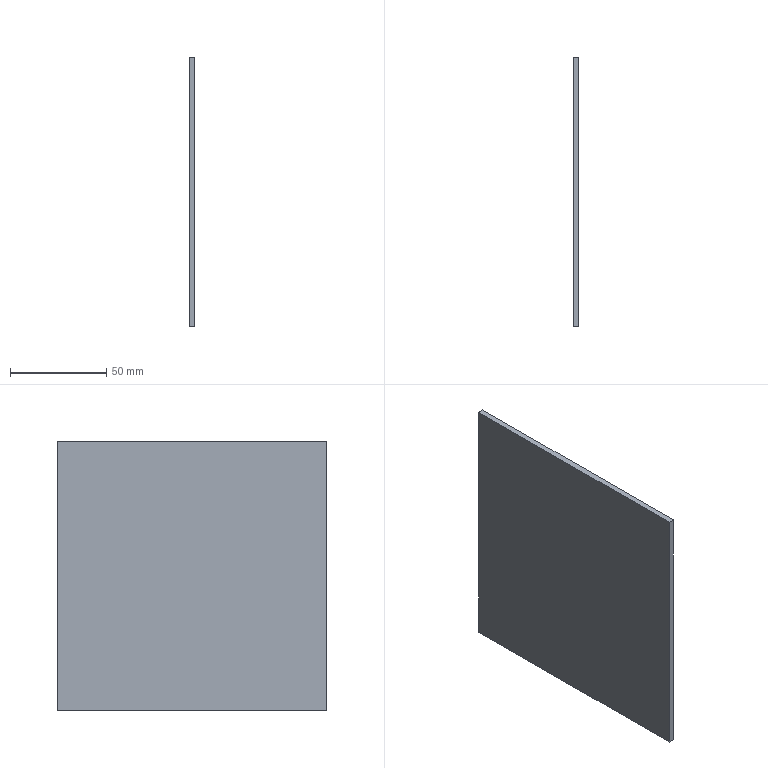Part | STEP file | Positioning_id1514_x_t | 1 solid | 6 faces | box 3 x 140 x 140 mm | volume 58800 mm3 | plane 6
STEP:
#1=CARTESIAN_POINT('',(0.,0.,0.));
#2=DIRECTION('',(0.,0.,1.));
#3=DIRECTION('',(1.,0.,0.));
#4=AXIS2_PLACEMENT_3D('',#1,#2,#3);
#5=CARTESIAN_POINT('',(-1013.002,-340.,368.995));
#6=VERTEX_POINT('',#5);
#7=CARTESIAN_POINT('',(-1010.002,-340.,368.995));
#8=VERTEX_POINT('',#7);
#9=CARTESIAN_POINT('',(-1013.002,-340.,368.995));
#10=DIRECTION('',(1.,0.,0.));
#11=VECTOR('',#10,1.);
#12=LINE('',#9,#11);
#13=CARTESIAN_POINT('',(-1018.002,-340.,283.995));
#14=DIRECTION('',(0.,1.,0.));
#15=DIRECTION('',(1.,0.,0.));
#16=AXIS2_PLACEMENT_3D('',#13,#14,#15);
#17=PLANE('',#16);
#18=CARTESIAN_POINT('',(5.,-85.));
#19=DIRECTION('',(1.,0.));
#20=VECTOR('',#19,1.);
#21=LINE('',#18,#20);
#22=(GEOMETRIC_REPRESENTATION_CONTEXT(2)PARAMETRIC_REPRESENTATION_CONTEXT()REPRESENTATION_CONTEXT('',''));
#23=DEFINITIONAL_REPRESENTATION('',(#21),#22);
#24=PCURVE('',#17,#23);
#25=CARTESIAN_POINT('',(-1018.002,-428.,368.995));
#26=DIRECTION('',(0.,0.,1.));
#27=DIRECTION('',(1.,0.,0.));
#28=AXIS2_PLACEMENT_3D('',#25,#26,#27);
#29=PLANE('',#28);
#30=CARTESIAN_POINT('',(5.,88.));
#31=DIRECTION('',(1.,0.));
#32=VECTOR('',#31,1.);
#33=LINE('',#30,#32);
#34=(GEOMETRIC_REPRESENTATION_CONTEXT(2)PARAMETRIC_REPRESENTATION_CONTEXT()REPRESENTATION_CONTEXT('',''));
#35=DEFINITIONAL_REPRESENTATION('',(#33),#34);
#36=PCURVE('',#29,#35);
#37=SURFACE_CURVE('',#12,(#24,#36),.PCURVE_S1.);
#38=EDGE_CURVE('',#6,#8,#37,.T.);
#39=ORIENTED_EDGE('',*,*,#38,.T.);
#40=CARTESIAN_POINT('',(-1010.002,-340.,228.995));
#41=VERTEX_POINT('',#40);
#42=CARTESIAN_POINT('',(-1010.002,-340.,368.995));
#43=DIRECTION('',(0.,0.,-1.));
#44=VECTOR('',#43,1.);
#45=LINE('',#42,#44);
#46=CARTESIAN_POINT('',(8.,-85.));
#47=DIRECTION('',(0.,1.));
#48=VECTOR('',#47,1.);
#49=LINE('',#46,#48);
#50=(GEOMETRIC_REPRESENTATION_CONTEXT(2)PARAMETRIC_REPRESENTATION_CONTEXT()REPRESENTATION_CONTEXT('',''));
#51=DEFINITIONAL_REPRESENTATION('',(#49),#50);
#52=PCURVE('',#17,#51);
#53=CARTESIAN_POINT('',(-1010.002,-480.,368.995));
#54=DIRECTION('',(1.,0.,0.));
#55=DIRECTION('',(0.,0.,-1.));
#56=AXIS2_PLACEMENT_3D('',#53,#54,#55);
#57=PLANE('',#56);
#58=CARTESIAN_POINT('',(0.,140.));
#59=DIRECTION('',(1.,0.));
#60=VECTOR('',#59,1.);
#61=LINE('',#58,#60);
#62=(GEOMETRIC_REPRESENTATION_CONTEXT(2)PARAMETRIC_REPRESENTATION_CONTEXT()REPRESENTATION_CONTEXT('',''));
#63=DEFINITIONAL_REPRESENTATION('',(#61),#62);
#64=PCURVE('',#57,#63);
#65=SURFACE_CURVE('',#45,(#52,#64),.PCURVE_S1.);
#66=EDGE_CURVE('',#8,#41,#65,.T.);
#67=ORIENTED_EDGE('',*,*,#66,.T.);
#68=CARTESIAN_POINT('',(-1013.002,-340.,228.995));
#69=VERTEX_POINT('',#68);
#70=CARTESIAN_POINT('',(-1013.002,-340.,228.995));
#71=DIRECTION('',(1.,0.,0.));
#72=VECTOR('',#71,1.);
#73=LINE('',#70,#72);
#74=CARTESIAN_POINT('',(5.,55.));
#75=DIRECTION('',(1.,0.));
#76=VECTOR('',#75,1.);
#77=LINE('',#74,#76);
#78=(GEOMETRIC_REPRESENTATION_CONTEXT(2)PARAMETRIC_REPRESENTATION_CONTEXT()REPRESENTATION_CONTEXT('',''));
#79=DEFINITIONAL_REPRESENTATION('',(#77),#78);
#80=PCURVE('',#17,#79);
#81=CARTESIAN_POINT('',(-1018.002,-428.,228.995));
#82=DIRECTION('',(0.,0.,-1.));
#83=DIRECTION('',(-1.,0.,0.));
#84=AXIS2_PLACEMENT_3D('',#81,#82,#83);
#85=PLANE('',#84);
#86=CARTESIAN_POINT('',(-5.,88.));
#87=DIRECTION('',(-1.,0.));
#88=VECTOR('',#87,1.);
#89=LINE('',#86,#88);
#90=(GEOMETRIC_REPRESENTATION_CONTEXT(2)PARAMETRIC_REPRESENTATION_CONTEXT()REPRESENTATION_CONTEXT('',''));
#91=DEFINITIONAL_REPRESENTATION('',(#89),#90);
#92=PCURVE('',#85,#91);
#93=SURFACE_CURVE('',#73,(#80,#92),.PCURVE_S1.);
#94=EDGE_CURVE('',#69,#41,#93,.T.);
#95=ORIENTED_EDGE('',*,*,#94,.F.);
#96=CARTESIAN_POINT('',(-1013.002,-340.,228.995));
#97=DIRECTION('',(0.,0.,1.));
#98=VECTOR('',#97,1.);
#99=LINE('',#96,#98);
#100=CARTESIAN_POINT('',(5.,55.));
#101=DIRECTION('',(0.,-1.));
#102=VECTOR('',#101,1.);
#103=LINE('',#100,#102);
#104=(GEOMETRIC_REPRESENTATION_CONTEXT(2)PARAMETRIC_REPRESENTATION_CONTEXT()REPRESENTATION_CONTEXT('',''));
#105=DEFINITIONAL_REPRESENTATION('',(#103),#104);
#106=PCURVE('',#17,#105);
#107=CARTESIAN_POINT('',(-1013.002,-428.,283.995));
#108=DIRECTION('',(-1.,0.,0.));
#109=DIRECTION('',(0.,0.,1.));
#110=AXIS2_PLACEMENT_3D('',#107,#108,#109);
#111=PLANE('',#110);
#112=CARTESIAN_POINT('',(-55.,88.));
#113=DIRECTION('',(1.,0.));
#114=VECTOR('',#113,1.);
#115=LINE('',#112,#114);
#116=(GEOMETRIC_REPRESENTATION_CONTEXT(2)PARAMETRIC_REPRESENTATION_CONTEXT()REPRESENTATION_CONTEXT('',''));
#117=DEFINITIONAL_REPRESENTATION('',(#115),#116);
#118=PCURVE('',#111,#117);
#119=SURFACE_CURVE('',#99,(#106,#118),.PCURVE_S1.);
#120=EDGE_CURVE('',#69,#6,#119,.T.);
#121=ORIENTED_EDGE('',*,*,#120,.T.);
#122=EDGE_LOOP('',(#39,#67,#95,#121));
#123=FACE_BOUND('',#122,.T.);
#124=ADVANCED_FACE('',(#123),#17,.T.);
#125=ORIENTED_EDGE('',*,*,#94,.T.);
#126=CARTESIAN_POINT('',(-1010.002,-480.,228.995));
#127=VERTEX_POINT('',#126);
#128=CARTESIAN_POINT('',(-1010.002,-340.,228.995));
#129=DIRECTION('',(0.,-1.,0.));
#130=VECTOR('',#129,1.);
#131=LINE('',#128,#130);
#132=CARTESIAN_POINT('',(-8.,88.));
#133=DIRECTION('',(0.,-1.));
#134=VECTOR('',#133,1.);
#135=LINE('',#132,#134);
#136=(GEOMETRIC_REPRESENTATION_CONTEXT(2)PARAMETRIC_REPRESENTATION_CONTEXT()REPRESENTATION_CONTEXT('',''));
#137=DEFINITIONAL_REPRESENTATION('',(#135),#136);
#138=PCURVE('',#85,#137);
#139=CARTESIAN_POINT('',(140.,140.));
#140=DIRECTION('',(0.,-1.));
#141=VECTOR('',#140,1.);
#142=LINE('',#139,#141);
#143=(GEOMETRIC_REPRESENTATION_CONTEXT(2)PARAMETRIC_REPRESENTATION_CONTEXT()REPRESENTATION_CONTEXT('',''));
#144=DEFINITIONAL_REPRESENTATION('',(#142),#143);
#145=PCURVE('',#57,#144);
#146=SURFACE_CURVE('',#131,(#138,#145),.PCURVE_S1.);
#147=EDGE_CURVE('',#41,#127,#146,.T.);
#148=ORIENTED_EDGE('',*,*,#147,.T.);
#149=CARTESIAN_POINT('',(-1013.002,-480.,228.995));
#150=VERTEX_POINT('',#149);
#151=CARTESIAN_POINT('',(-1013.002,-480.,228.995));
#152=DIRECTION('',(1.,0.,0.));
#153=VECTOR('',#152,1.);
#154=LINE('',#151,#153);
#155=CARTESIAN_POINT('',(-5.,-52.));
#156=DIRECTION('',(-1.,0.));
#157=VECTOR('',#156,1.);
#158=LINE('',#155,#157);
#159=(GEOMETRIC_REPRESENTATION_CONTEXT(2)PARAMETRIC_REPRESENTATION_CONTEXT()REPRESENTATION_CONTEXT('',''));
#160=DEFINITIONAL_REPRESENTATION('',(#158),#159);
#161=PCURVE('',#85,#160);
#162=CARTESIAN_POINT('',(-1018.002,-480.,283.995));
#163=DIRECTION('',(0.,-1.,0.));
#164=DIRECTION('',(-1.,0.,0.));
#165=AXIS2_PLACEMENT_3D('',#162,#163,#164);
#166=PLANE('',#165);
#167=CARTESIAN_POINT('',(-5.,55.));
#168=DIRECTION('',(-1.,0.));
#169=VECTOR('',#168,1.);
#170=LINE('',#167,#169);
#171=(GEOMETRIC_REPRESENTATION_CONTEXT(2)PARAMETRIC_REPRESENTATION_CONTEXT()REPRESENTATION_CONTEXT('',''));
#172=DEFINITIONAL_REPRESENTATION('',(#170),#171);
#173=PCURVE('',#166,#172);
#174=SURFACE_CURVE('',#154,(#161,#173),.PCURVE_S1.);
#175=EDGE_CURVE('',#150,#127,#174,.T.);
#176=ORIENTED_EDGE('',*,*,#175,.F.);
#177=CARTESIAN_POINT('',(-1013.002,-480.,228.995));
#178=DIRECTION('',(0.,1.,0.));
#179=VECTOR('',#178,1.);
#180=LINE('',#177,#179);
#181=CARTESIAN_POINT('',(-5.,-52.));
#182=DIRECTION('',(0.,1.));
#183=VECTOR('',#182,1.);
#184=LINE('',#181,#183);
#185=(GEOMETRIC_REPRESENTATION_CONTEXT(2)PARAMETRIC_REPRESENTATION_CONTEXT()REPRESENTATION_CONTEXT('',''));
#186=DEFINITIONAL_REPRESENTATION('',(#184),#185);
#187=PCURVE('',#85,#186);
#188=CARTESIAN_POINT('',(-55.,-52.));
#189=DIRECTION('',(0.,1.));
#190=VECTOR('',#189,1.);
#191=LINE('',#188,#190);
#192=(GEOMETRIC_REPRESENTATION_CONTEXT(2)PARAMETRIC_REPRESENTATION_CONTEXT()REPRESENTATION_CONTEXT('',''));
#193=DEFINITIONAL_REPRESENTATION('',(#191),#192);
#194=PCURVE('',#111,#193);
#195=SURFACE_CURVE('',#180,(#187,#194),.PCURVE_S1.);
#196=EDGE_CURVE('',#150,#69,#195,.T.);
#197=ORIENTED_EDGE('',*,*,#196,.T.);
#198=EDGE_LOOP('',(#125,#148,#176,#197));
#199=FACE_BOUND('',#198,.T.);
#200=ADVANCED_FACE('',(#199),#85,.T.);
#201=ORIENTED_EDGE('',*,*,#175,.T.);
#202=CARTESIAN_POINT('',(-1010.002,-480.,368.995));
#203=VERTEX_POINT('',#202);
#204=CARTESIAN_POINT('',(-1010.002,-480.,228.995));
#205=DIRECTION('',(0.,0.,1.));
#206=VECTOR('',#205,1.);
#207=LINE('',#204,#206);
#208=CARTESIAN_POINT('',(-8.,55.));
#209=DIRECTION('',(0.,-1.));
#210=VECTOR('',#209,1.);
#211=LINE('',#208,#210);
#212=(GEOMETRIC_REPRESENTATION_CONTEXT(2)PARAMETRIC_REPRESENTATION_CONTEXT()REPRESENTATION_CONTEXT('',''));
#213=DEFINITIONAL_REPRESENTATION('',(#211),#212);
#214=PCURVE('',#166,#213);
#215=CARTESIAN_POINT('',(140.,0.));
#216=DIRECTION('',(-1.,0.));
#217=VECTOR('',#216,1.);
#218=LINE('',#215,#217);
#219=(GEOMETRIC_REPRESENTATION_CONTEXT(2)PARAMETRIC_REPRESENTATION_CONTEXT()REPRESENTATION_CONTEXT('',''));
#220=DEFINITIONAL_REPRESENTATION('',(#218),#219);
#221=PCURVE('',#57,#220);
#222=SURFACE_CURVE('',#207,(#214,#221),.PCURVE_S1.);
#223=EDGE_CURVE('',#127,#203,#222,.T.);
#224=ORIENTED_EDGE('',*,*,#223,.T.);
#225=CARTESIAN_POINT('',(-1013.002,-480.,368.995));
#226=VERTEX_POINT('',#225);
#227=CARTESIAN_POINT('',(-1013.002,-480.,368.995));
#228=DIRECTION('',(1.,0.,0.));
#229=VECTOR('',#228,1.);
#230=LINE('',#227,#229);
#231=CARTESIAN_POINT('',(-5.,-85.));
#232=DIRECTION('',(-1.,0.));
#233=VECTOR('',#232,1.);
#234=LINE('',#231,#233);
#235=(GEOMETRIC_REPRESENTATION_CONTEXT(2)PARAMETRIC_REPRESENTATION_CONTEXT()REPRESENTATION_CONTEXT('',''));
#236=DEFINITIONAL_REPRESENTATION('',(#234),#235);
#237=PCURVE('',#166,#236);
#238=CARTESIAN_POINT('',(5.,-52.));
#239=DIRECTION('',(1.,0.));
#240=VECTOR('',#239,1.);
#241=LINE('',#238,#240);
#242=(GEOMETRIC_REPRESENTATION_CONTEXT(2)PARAMETRIC_REPRESENTATION_CONTEXT()REPRESENTATION_CONTEXT('',''));
#243=DEFINITIONAL_REPRESENTATION('',(#241),#242);
#244=PCURVE('',#29,#243);
#245=SURFACE_CURVE('',#230,(#237,#244),.PCURVE_S1.);
#246=EDGE_CURVE('',#226,#203,#245,.T.);
#247=ORIENTED_EDGE('',*,*,#246,.F.);
#248=CARTESIAN_POINT('',(-1013.002,-480.,368.995));
#249=DIRECTION('',(0.,0.,-1.));
#250=VECTOR('',#249,1.);
#251=LINE('',#248,#250);
#252=CARTESIAN_POINT('',(-5.,-85.));
#253=DIRECTION('',(0.,1.));
#254=VECTOR('',#253,1.);
#255=LINE('',#252,#254);
#256=(GEOMETRIC_REPRESENTATION_CONTEXT(2)PARAMETRIC_REPRESENTATION_CONTEXT()REPRESENTATION_CONTEXT('',''));
#257=DEFINITIONAL_REPRESENTATION('',(#255),#256);
#258=PCURVE('',#166,#257);
#259=CARTESIAN_POINT('',(85.,-52.));
#260=DIRECTION('',(-1.,0.));
#261=VECTOR('',#260,1.);
#262=LINE('',#259,#261);
#263=(GEOMETRIC_REPRESENTATION_CONTEXT(2)PARAMETRIC_REPRESENTATION_CONTEXT()REPRESENTATION_CONTEXT('',''));
#264=DEFINITIONAL_REPRESENTATION('',(#262),#263);
#265=PCURVE('',#111,#264);
#266=SURFACE_CURVE('',#251,(#258,#265),.PCURVE_S1.);
#267=EDGE_CURVE('',#226,#150,#266,.T.);
#268=ORIENTED_EDGE('',*,*,#267,.T.);
#269=EDGE_LOOP('',(#201,#224,#247,#268));
#270=FACE_BOUND('',#269,.T.);
#271=ADVANCED_FACE('',(#270),#166,.T.);
#272=ORIENTED_EDGE('',*,*,#246,.T.);
#273=CARTESIAN_POINT('',(-1010.002,-480.,368.995));
#274=DIRECTION('',(0.,1.,0.));
#275=VECTOR('',#274,1.);
#276=LINE('',#273,#275);
#277=CARTESIAN_POINT('',(8.,-52.));
#278=DIRECTION('',(0.,1.));
#279=VECTOR('',#278,1.);
#280=LINE('',#277,#279);
#281=(GEOMETRIC_REPRESENTATION_CONTEXT(2)PARAMETRIC_REPRESENTATION_CONTEXT()REPRESENTATION_CONTEXT('',''));
#282=DEFINITIONAL_REPRESENTATION('',(#280),#281);
#283=PCURVE('',#29,#282);
#284=CARTESIAN_POINT('',(0.,0.));
#285=DIRECTION('',(0.,1.));
#286=VECTOR('',#285,1.);
#287=LINE('',#284,#286);
#288=(GEOMETRIC_REPRESENTATION_CONTEXT(2)PARAMETRIC_REPRESENTATION_CONTEXT()REPRESENTATION_CONTEXT('',''));
#289=DEFINITIONAL_REPRESENTATION('',(#287),#288);
#290=PCURVE('',#57,#289);
#291=SURFACE_CURVE('',#276,(#283,#290),.PCURVE_S1.);
#292=EDGE_CURVE('',#203,#8,#291,.T.);
#293=ORIENTED_EDGE('',*,*,#292,.T.);
#294=ORIENTED_EDGE('',*,*,#38,.F.);
#295=CARTESIAN_POINT('',(-1013.002,-340.,368.995));
#296=DIRECTION('',(0.,-1.,0.));
#297=VECTOR('',#296,1.);
#298=LINE('',#295,#297);
#299=CARTESIAN_POINT('',(5.,88.));
#300=DIRECTION('',(0.,-1.));
#301=VECTOR('',#300,1.);
#302=LINE('',#299,#301);
#303=(GEOMETRIC_REPRESENTATION_CONTEXT(2)PARAMETRIC_REPRESENTATION_CONTEXT()REPRESENTATION_CONTEXT('',''));
#304=DEFINITIONAL_REPRESENTATION('',(#302),#303);
#305=PCURVE('',#29,#304);
#306=CARTESIAN_POINT('',(85.,88.));
#307=DIRECTION('',(0.,-1.));
#308=VECTOR('',#307,1.);
#309=LINE('',#306,#308);
#310=(GEOMETRIC_REPRESENTATION_CONTEXT(2)PARAMETRIC_REPRESENTATION_CONTEXT()REPRESENTATION_CONTEXT('',''));
#311=DEFINITIONAL_REPRESENTATION('',(#309),#310);
#312=PCURVE('',#111,#311);
#313=SURFACE_CURVE('',#298,(#305,#312),.PCURVE_S1.);
#314=EDGE_CURVE('',#6,#226,#313,.T.);
#315=ORIENTED_EDGE('',*,*,#314,.T.);
#316=EDGE_LOOP('',(#272,#293,#294,#315));
#317=FACE_BOUND('',#316,.T.);
#318=ADVANCED_FACE('',(#317),#29,.T.);
#319=ORIENTED_EDGE('',*,*,#314,.F.);
#320=ORIENTED_EDGE('',*,*,#120,.F.);
#321=ORIENTED_EDGE('',*,*,#196,.F.);
#322=ORIENTED_EDGE('',*,*,#267,.F.);
#323=EDGE_LOOP('',(#319,#320,#321,#322));
#324=FACE_BOUND('',#323,.T.);
#325=ADVANCED_FACE('',(#324),#111,.T.);
#326=ORIENTED_EDGE('',*,*,#66,.F.);
#327=ORIENTED_EDGE('',*,*,#292,.F.);
#328=ORIENTED_EDGE('',*,*,#223,.F.);
#329=ORIENTED_EDGE('',*,*,#147,.F.);
#330=EDGE_LOOP('',(#326,#327,#328,#329));
#331=FACE_BOUND('',#330,.T.);
#332=ADVANCED_FACE('',(#331),#57,.T.);
#333=CLOSED_SHELL('',(#124,#200,#271,#318,#325,#332));
#334=MANIFOLD_SOLID_BREP('',#333);
#335=(LENGTH_UNIT()NAMED_UNIT(*)SI_UNIT(.MILLI.,.METRE.));
#336=UNCERTAINTY_MEASURE_WITH_UNIT(LENGTH_MEASURE(0.0000001),#335,'','');
#337=(NAMED_UNIT(*)PLANE_ANGLE_UNIT()SI_UNIT($,.RADIAN.));
#338=(NAMED_UNIT(*)SI_UNIT($,.STERADIAN.)SOLID_ANGLE_UNIT());
#339=(GEOMETRIC_REPRESENTATION_CONTEXT(3)GLOBAL_UNCERTAINTY_ASSIGNED_CONTEXT((#336))GLOBAL_UNIT_ASSIGNED_CONTEXT((#335,#337,#338))REPRESENTATION_CONTEXT('',''));
#340=ADVANCED_BREP_SHAPE_REPRESENTATION('',(#4,#334),#339);